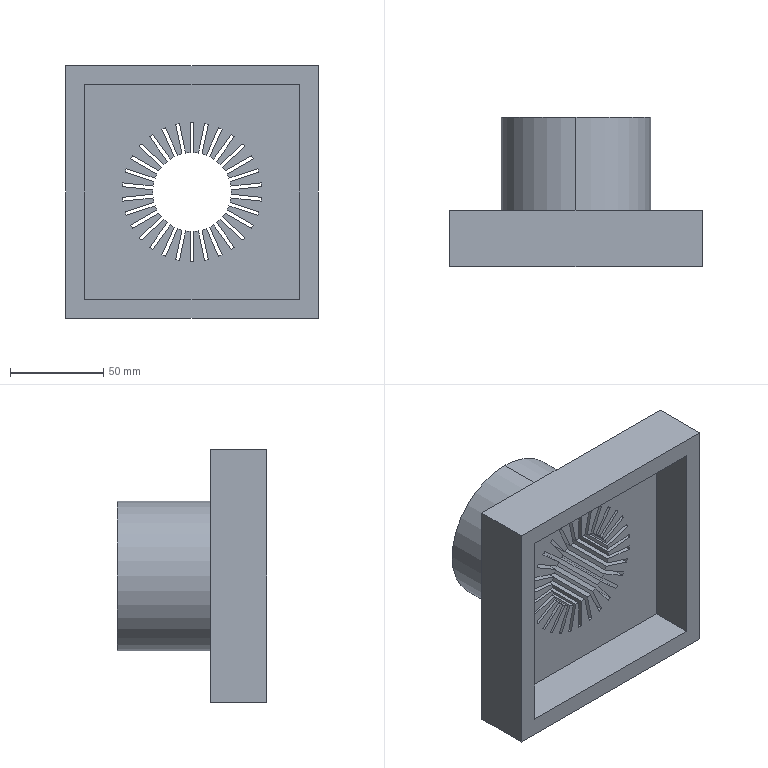Part | SolidWorks | features BaseBody 1 | 1 solid | 135 faces | box 135 x 80 x 135 mm | volume 358960 mm3 | plane 72 | cylinder 63 | commonest cylinder face diameters 74.485 x31 42.2 x30 80 x2